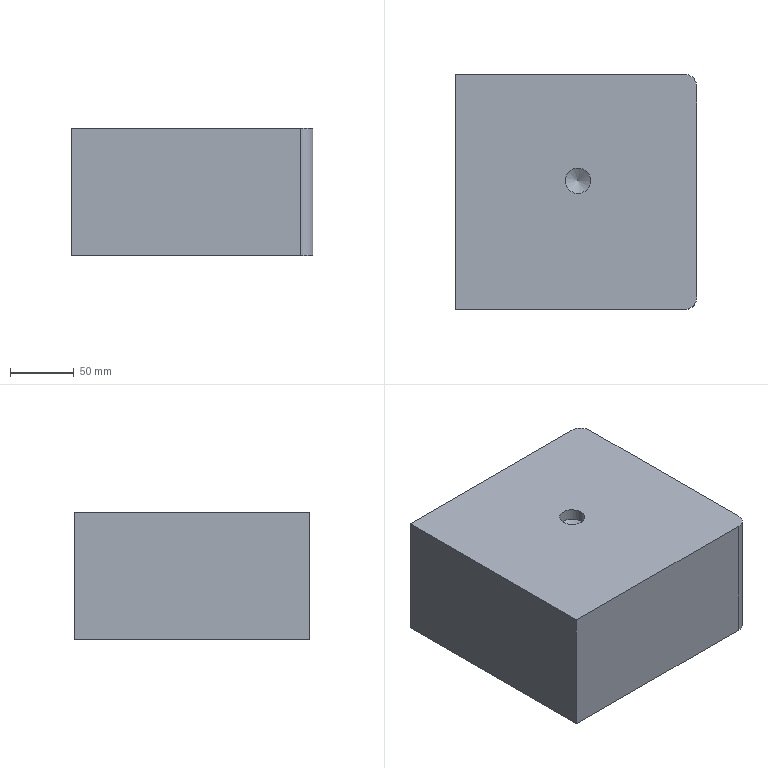Part | NX | features solid 2 | 1 solid | 10 faces | box 190 x 185 x 100 mm | volume 3507251 mm3 | plane 6 | cylinder 3 | cone 1 | commonest cylinder face diameters 20 x3
STEP:
#1=CARTESIAN_POINT('',(-620.,-125.,-320.));
#2=VERTEX_POINT('',#1);
#3=CARTESIAN_POINT('',(-440.,-125.,-320.));
#4=VERTEX_POINT('',#3);
#5=CARTESIAN_POINT('',(-620.,-125.,-320.));
#6=DIRECTION('',(-1.,0.,0.));
#7=VECTOR('',#6,1000.);
#8=LINE('',#5,#7);
#9=EDGE_CURVE('',#2,#4,#8,.F.);
#10=ORIENTED_EDGE('',*,*,#9,.T.);
#11=CARTESIAN_POINT('',(-430.,-135.,-320.));
#12=VERTEX_POINT('',#11);
#13=CARTESIAN_POINT('',(-440.,-135.,-320.));
#14=DIRECTION('',(0.,0.,-1.));
#15=DIRECTION('',(-1.,0.,0.));
#16=AXIS2_PLACEMENT_3D('',#13,#14,#15);
#17=CIRCLE('',#16,10.);
#18=EDGE_CURVE('',#4,#12,#17,.T.);
#19=ORIENTED_EDGE('',*,*,#18,.T.);
#20=CARTESIAN_POINT('',(-430.,-300.,-320.));
#21=VERTEX_POINT('',#20);
#22=CARTESIAN_POINT('',(-430.,-125.,-320.));
#23=DIRECTION('',(0.,1.,0.));
#24=VECTOR('',#23,1000.);
#25=LINE('',#22,#24);
#26=EDGE_CURVE('',#12,#21,#25,.F.);
#27=ORIENTED_EDGE('',*,*,#26,.T.);
#28=CARTESIAN_POINT('',(-440.,-310.,-320.));
#29=VERTEX_POINT('',#28);
#30=CARTESIAN_POINT('',(-440.,-300.,-320.));
#31=DIRECTION('',(0.,0.,-1.));
#32=DIRECTION('',(-1.,0.,0.));
#33=AXIS2_PLACEMENT_3D('',#30,#31,#32);
#34=CIRCLE('',#33,10.);
#35=EDGE_CURVE('',#21,#29,#34,.T.);
#36=ORIENTED_EDGE('',*,*,#35,.T.);
#37=CARTESIAN_POINT('',(-620.,-310.,-320.));
#38=VERTEX_POINT('',#37);
#39=CARTESIAN_POINT('',(-620.,-310.,-320.));
#40=DIRECTION('',(-1.,0.,0.));
#41=VECTOR('',#40,1000.);
#42=LINE('',#39,#41);
#43=EDGE_CURVE('',#38,#29,#42,.F.);
#44=ORIENTED_EDGE('',*,*,#43,.F.);
#45=CARTESIAN_POINT('',(-620.,-125.,-320.));
#46=DIRECTION('',(0.,-1.,0.));
#47=VECTOR('',#46,1000.);
#48=LINE('',#45,#47);
#49=EDGE_CURVE('',#2,#38,#48,.T.);
#50=ORIENTED_EDGE('',*,*,#49,.F.);
#51=EDGE_LOOP('',(#10,#19,#27,#36,#44,#50));
#52=FACE_BOUND('',#51,.T.);
#53=CARTESIAN_POINT('',(-620.,-125.,-320.));
#54=DIRECTION('',(0.,0.,-1.));
#55=DIRECTION('',(0.,-1.,0.));
#56=AXIS2_PLACEMENT_3D('',#53,#54,#55);
#57=PLANE('',#56);
#58=ADVANCED_FACE('',(#52),#57,.T.);
#59=ORIENTED_EDGE('',*,*,#43,.T.);
#60=CARTESIAN_POINT('',(-440.,-310.,-220.));
#61=VERTEX_POINT('',#60);
#62=CARTESIAN_POINT('',(-440.,-310.,-320.));
#63=DIRECTION('',(0.,0.,1.));
#64=VECTOR('',#63,1000.);
#65=LINE('',#62,#64);
#66=EDGE_CURVE('',#29,#61,#65,.T.);
#67=ORIENTED_EDGE('',*,*,#66,.T.);
#68=CARTESIAN_POINT('',(-620.,-310.,-220.));
#69=VERTEX_POINT('',#68);
#70=CARTESIAN_POINT('',(-620.,-310.,-220.));
#71=DIRECTION('',(-1.,0.,0.));
#72=VECTOR('',#71,1000.);
#73=LINE('',#70,#72);
#74=EDGE_CURVE('',#69,#61,#73,.F.);
#75=ORIENTED_EDGE('',*,*,#74,.F.);
#76=CARTESIAN_POINT('',(-620.,-310.,-320.));
#77=DIRECTION('',(0.,0.,1.));
#78=VECTOR('',#77,1000.);
#79=LINE('',#76,#78);
#80=EDGE_CURVE('',#38,#69,#79,.T.);
#81=ORIENTED_EDGE('',*,*,#80,.F.);
#82=EDGE_LOOP('',(#59,#67,#75,#81));
#83=FACE_BOUND('',#82,.T.);
#84=CARTESIAN_POINT('',(-620.,-310.,-320.));
#85=DIRECTION('',(0.,-1.,0.));
#86=DIRECTION('',(0.,0.,1.));
#87=AXIS2_PLACEMENT_3D('',#84,#85,#86);
#88=PLANE('',#87);
#89=ADVANCED_FACE('',(#83),#88,.T.);
#90=CARTESIAN_POINT('',(-533.47,-208.789,-220.));
#91=VERTEX_POINT('',#90);
#92=CARTESIAN_POINT('',(-523.47,-208.789,-220.));
#93=DIRECTION('',(0.,0.,-1.));
#94=DIRECTION('',(-1.,0.,0.));
#95=AXIS2_PLACEMENT_3D('',#92,#93,#94);
#96=CIRCLE('',#95,10.);
#97=EDGE_CURVE('',#91,#91,#96,.T.);
#98=ORIENTED_EDGE('',*,*,#97,.T.);
#99=EDGE_LOOP('',(#98));
#100=FACE_BOUND('',#99,.T.);
#101=CARTESIAN_POINT('',(-430.,-135.,-220.));
#102=VERTEX_POINT('',#101);
#103=CARTESIAN_POINT('',(-430.,-300.,-220.));
#104=VERTEX_POINT('',#103);
#105=CARTESIAN_POINT('',(-430.,-125.,-220.));
#106=DIRECTION('',(0.,1.,0.));
#107=VECTOR('',#106,1000.);
#108=LINE('',#105,#107);
#109=EDGE_CURVE('',#102,#104,#108,.F.);
#110=ORIENTED_EDGE('',*,*,#109,.F.);
#111=CARTESIAN_POINT('',(-440.,-125.,-220.));
#112=VERTEX_POINT('',#111);
#113=CARTESIAN_POINT('',(-440.,-135.,-220.));
#114=DIRECTION('',(0.,0.,-1.));
#115=DIRECTION('',(-1.,0.,0.));
#116=AXIS2_PLACEMENT_3D('',#113,#114,#115);
#117=CIRCLE('',#116,10.);
#118=EDGE_CURVE('',#102,#112,#117,.F.);
#119=ORIENTED_EDGE('',*,*,#118,.T.);
#120=CARTESIAN_POINT('',(-620.,-125.,-220.));
#121=VERTEX_POINT('',#120);
#122=CARTESIAN_POINT('',(-620.,-125.,-220.));
#123=DIRECTION('',(-1.,0.,0.));
#124=VECTOR('',#123,1000.);
#125=LINE('',#122,#124);
#126=EDGE_CURVE('',#121,#112,#125,.F.);
#127=ORIENTED_EDGE('',*,*,#126,.F.);
#128=CARTESIAN_POINT('',(-620.,-125.,-220.));
#129=DIRECTION('',(0.,-1.,0.));
#130=VECTOR('',#129,1000.);
#131=LINE('',#128,#130);
#132=EDGE_CURVE('',#121,#69,#131,.T.);
#133=ORIENTED_EDGE('',*,*,#132,.T.);
#134=ORIENTED_EDGE('',*,*,#74,.T.);
#135=CARTESIAN_POINT('',(-440.,-300.,-220.));
#136=DIRECTION('',(0.,0.,-1.));
#137=DIRECTION('',(-1.,0.,0.));
#138=AXIS2_PLACEMENT_3D('',#135,#136,#137);
#139=CIRCLE('',#138,10.);
#140=EDGE_CURVE('',#61,#104,#139,.F.);
#141=ORIENTED_EDGE('',*,*,#140,.T.);
#142=EDGE_LOOP('',(#110,#119,#127,#133,#134,#141));
#143=FACE_BOUND('',#142,.T.);
#144=CARTESIAN_POINT('',(-620.,-125.,-220.));
#145=DIRECTION('',(0.,0.,-1.));
#146=DIRECTION('',(0.,-1.,0.));
#147=AXIS2_PLACEMENT_3D('',#144,#145,#146);
#148=PLANE('',#147);
#149=ADVANCED_FACE('',(#100,#143),#148,.F.);
#150=ORIENTED_EDGE('',*,*,#126,.T.);
#151=CARTESIAN_POINT('',(-440.,-125.,-320.));
#152=DIRECTION('',(0.,0.,1.));
#153=VECTOR('',#152,1000.);
#154=LINE('',#151,#153);
#155=EDGE_CURVE('',#112,#4,#154,.F.);
#156=ORIENTED_EDGE('',*,*,#155,.T.);
#157=ORIENTED_EDGE('',*,*,#9,.F.);
#158=CARTESIAN_POINT('',(-620.,-125.,-320.));
#159=DIRECTION('',(0.,0.,1.));
#160=VECTOR('',#159,1000.);
#161=LINE('',#158,#160);
#162=EDGE_CURVE('',#2,#121,#161,.T.);
#163=ORIENTED_EDGE('',*,*,#162,.T.);
#164=EDGE_LOOP('',(#150,#156,#157,#163));
#165=FACE_BOUND('',#164,.T.);
#166=CARTESIAN_POINT('',(-620.,-125.,-320.));
#167=DIRECTION('',(0.,-1.,0.));
#168=DIRECTION('',(0.,0.,1.));
#169=AXIS2_PLACEMENT_3D('',#166,#167,#168);
#170=PLANE('',#169);
#171=ADVANCED_FACE('',(#165),#170,.F.);
#172=ORIENTED_EDGE('',*,*,#26,.F.);
#173=CARTESIAN_POINT('',(-430.,-135.,-320.));
#174=DIRECTION('',(0.,0.,1.));
#175=VECTOR('',#174,1000.);
#176=LINE('',#173,#175);
#177=EDGE_CURVE('',#12,#102,#176,.T.);
#178=ORIENTED_EDGE('',*,*,#177,.T.);
#179=ORIENTED_EDGE('',*,*,#109,.T.);
#180=CARTESIAN_POINT('',(-430.,-300.,-320.));
#181=DIRECTION('',(0.,0.,-1.));
#182=VECTOR('',#181,1000.);
#183=LINE('',#180,#182);
#184=EDGE_CURVE('',#104,#21,#183,.T.);
#185=ORIENTED_EDGE('',*,*,#184,.T.);
#186=EDGE_LOOP('',(#172,#178,#179,#185));
#187=FACE_BOUND('',#186,.T.);
#188=CARTESIAN_POINT('',(-430.,-125.,-320.));
#189=DIRECTION('',(-1.,0.,0.));
#190=DIRECTION('',(0.,0.,1.));
#191=AXIS2_PLACEMENT_3D('',#188,#189,#190);
#192=PLANE('',#191);
#193=ADVANCED_FACE('',(#187),#192,.F.);
#194=ORIENTED_EDGE('',*,*,#132,.F.);
#195=ORIENTED_EDGE('',*,*,#162,.F.);
#196=ORIENTED_EDGE('',*,*,#49,.T.);
#197=ORIENTED_EDGE('',*,*,#80,.T.);
#198=EDGE_LOOP('',(#194,#195,#196,#197));
#199=FACE_BOUND('',#198,.T.);
#200=CARTESIAN_POINT('',(-620.,-125.,-320.));
#201=DIRECTION('',(-1.,0.,0.));
#202=DIRECTION('',(0.,0.,1.));
#203=AXIS2_PLACEMENT_3D('',#200,#201,#202);
#204=PLANE('',#203);
#205=ADVANCED_FACE('',(#199),#204,.T.);
#206=ORIENTED_EDGE('',*,*,#18,.F.);
#207=ORIENTED_EDGE('',*,*,#155,.F.);
#208=ORIENTED_EDGE('',*,*,#118,.F.);
#209=ORIENTED_EDGE('',*,*,#177,.F.);
#210=EDGE_LOOP('',(#206,#207,#208,#209));
#211=FACE_BOUND('',#210,.T.);
#212=CARTESIAN_POINT('',(-440.,-135.,-320.));
#213=DIRECTION('',(0.,0.,1.));
#214=DIRECTION('',(1.,0.,0.));
#215=AXIS2_PLACEMENT_3D('',#212,#213,#214);
#216=CYLINDRICAL_SURFACE('',#215,10.);
#217=ADVANCED_FACE('',(#211),#216,.T.);
#218=ORIENTED_EDGE('',*,*,#35,.F.);
#219=ORIENTED_EDGE('',*,*,#184,.F.);
#220=ORIENTED_EDGE('',*,*,#140,.F.);
#221=ORIENTED_EDGE('',*,*,#66,.F.);
#222=EDGE_LOOP('',(#218,#219,#220,#221));
#223=FACE_BOUND('',#222,.T.);
#224=CARTESIAN_POINT('',(-440.,-300.,-320.));
#225=DIRECTION('',(0.,0.,-1.));
#226=DIRECTION('',(-1.,0.,0.));
#227=AXIS2_PLACEMENT_3D('',#224,#225,#226);
#228=CYLINDRICAL_SURFACE('',#227,10.);
#229=ADVANCED_FACE('',(#223),#228,.T.);
#230=CARTESIAN_POINT('',(-533.47,-208.789,-229.));
#231=VERTEX_POINT('',#230);
#232=CARTESIAN_POINT('',(-523.47,-208.789,-229.));
#233=DIRECTION('',(0.,0.,-1.));
#234=DIRECTION('',(-1.,0.,0.));
#235=AXIS2_PLACEMENT_3D('',#232,#233,#234);
#236=CIRCLE('',#235,10.);
#237=EDGE_CURVE('',#231,#231,#236,.F.);
#238=ORIENTED_EDGE('',*,*,#237,.T.);
#239=EDGE_LOOP('',(#238));
#240=FACE_BOUND('',#239,.T.);
#241=CARTESIAN_POINT('',(-523.47,-208.789,-235.009));
#242=VERTEX_POINT('',#241);
#243=VERTEX_LOOP('',#242);
#244=FACE_BOUND('',#243,.T.);
#245=CARTESIAN_POINT('',(-523.47,-208.789,-229.));
#246=DIRECTION('',(0.,0.,1.));
#247=DIRECTION('',(1.,0.,0.));
#248=AXIS2_PLACEMENT_3D('',#245,#246,#247);
#249=CONICAL_SURFACE('',#248,10.,1.03);
#250=ADVANCED_FACE('',(#240,#244),#249,.F.);
#251=ORIENTED_EDGE('',*,*,#237,.F.);
#252=EDGE_LOOP('',(#251));
#253=FACE_BOUND('',#252,.T.);
#254=ORIENTED_EDGE('',*,*,#97,.F.);
#255=EDGE_LOOP('',(#254));
#256=FACE_BOUND('',#255,.T.);
#257=CARTESIAN_POINT('',(-523.47,-208.789,-220.));
#258=DIRECTION('',(0.,0.,-1.));
#259=DIRECTION('',(-1.,0.,0.));
#260=AXIS2_PLACEMENT_3D('',#257,#258,#259);
#261=CYLINDRICAL_SURFACE('',#260,10.);
#262=ADVANCED_FACE('',(#253,#256),#261,.F.);
#263=CLOSED_SHELL('',(#58,#89,#149,#171,#193,#205,#217,#229,#250,#262));
#264=MANIFOLD_SOLID_BREP('',#263);
#265=(LENGTH_UNIT()NAMED_UNIT(*)SI_UNIT(.MILLI.,.METRE.));
#266=UNCERTAINTY_MEASURE_WITH_UNIT(LENGTH_MEASURE(0.00001),#265,'','');
#267=(NAMED_UNIT(*)PLANE_ANGLE_UNIT()SI_UNIT($,.RADIAN.));
#268=(NAMED_UNIT(*)SI_UNIT($,.STERADIAN.)SOLID_ANGLE_UNIT());
#269=(GEOMETRIC_REPRESENTATION_CONTEXT(3)GLOBAL_UNCERTAINTY_ASSIGNED_CONTEXT((#266))GLOBAL_UNIT_ASSIGNED_CONTEXT((#265,#267,#268))REPRESENTATION_CONTEXT('',''));
#270=ADVANCED_BREP_SHAPE_REPRESENTATION('',(#264),#269);